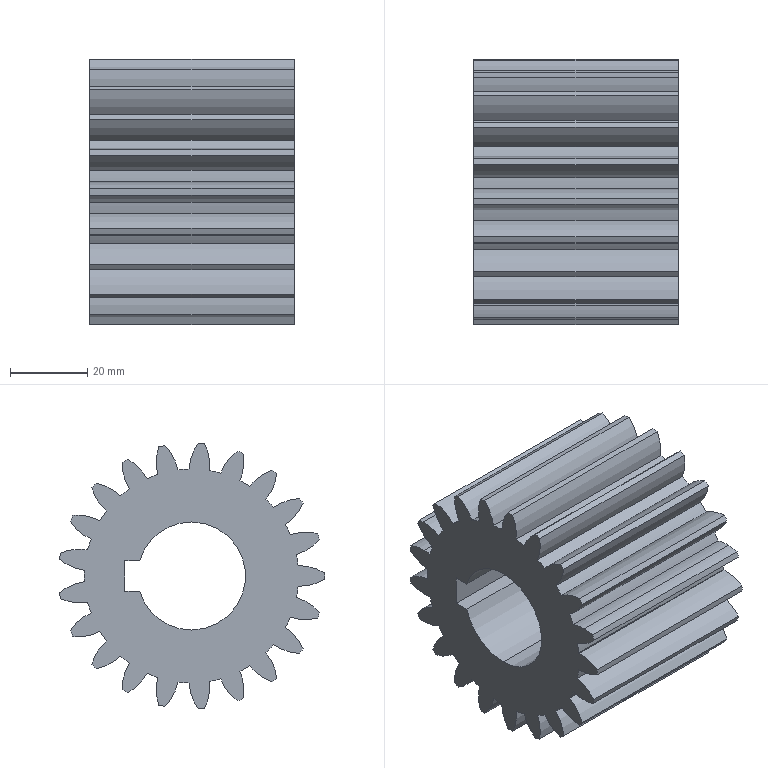Part | SolidWorks | features BaseBody 1, ICE 1 | 1 solid | 99 faces | box 53 x 68.725 x 68.909 mm | volume 123746 mm3 | cylinder 93 | plane 6 | commonest cylinder face diameters 25.2 x46 55.498 x21 69 x21 28 x3 36 x2